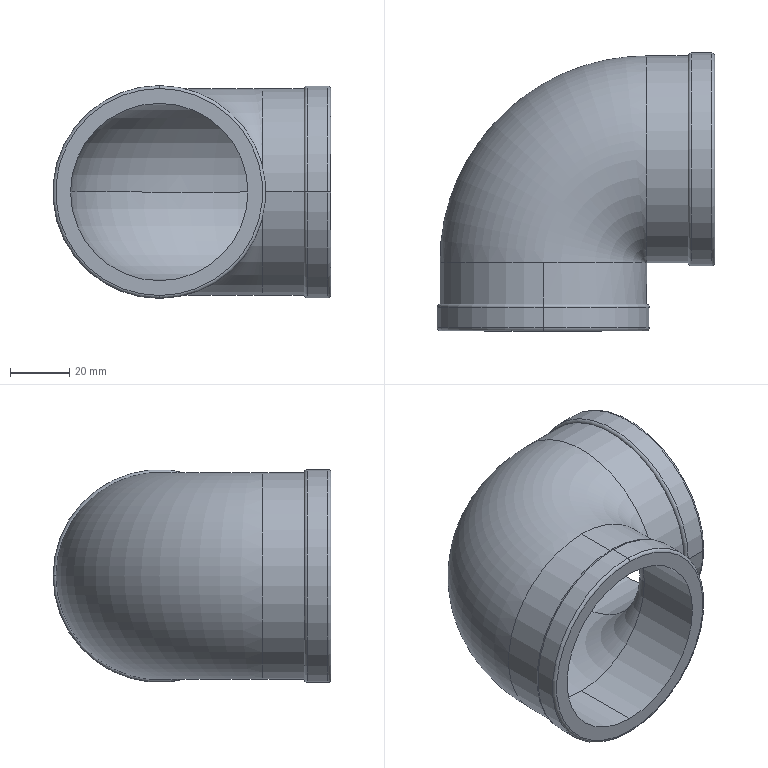Part | SolidWorks | features BossThin 2, Fillet 2, Sweep 1 | 1 solid | 25 faces | box 94 x 94 x 72 mm | volume 106922 mm3 | cylinder 12 | torus 11 | plane 2 | commonest cylinder face diameters 60 x4 70 x4 72 x4
STEP:
#1=CARTESIAN_POINT('',(-30.,23.,0.));
#2=VERTEX_POINT('',#1);
#3=CARTESIAN_POINT('',(0.,23.,30.));
#4=VERTEX_POINT('',#3);
#5=CARTESIAN_POINT('',(0.,23.,0.));
#6=DIRECTION('',(0.,1.,0.));
#7=DIRECTION('',(0.,0.,1.));
#8=AXIS2_PLACEMENT_3D('',#5,#6,#7);
#9=CIRCLE('',#8,30.);
#10=EDGE_CURVE('',#2,#4,#9,.T.);
#11=ORIENTED_EDGE('',*,*,#10,.F.);
#12=CARTESIAN_POINT('',(35.,88.,0.));
#13=VERTEX_POINT('',#12);
#14=CARTESIAN_POINT('',(35.,23.,0.));
#15=DIRECTION('',(0.,0.,-1.));
#16=DIRECTION('',(0.,1.,0.));
#17=AXIS2_PLACEMENT_3D('',#14,#15,#16);
#18=CIRCLE('',#17,65.);
#19=EDGE_CURVE('',#2,#13,#18,.T.);
#20=ORIENTED_EDGE('',*,*,#19,.T.);
#21=CARTESIAN_POINT('',(35.,28.,0.));
#22=VERTEX_POINT('',#21);
#23=CARTESIAN_POINT('',(35.,58.,0.));
#24=DIRECTION('',(1.,0.,0.));
#25=DIRECTION('',(0.,0.,1.));
#26=AXIS2_PLACEMENT_3D('',#23,#24,#25);
#27=CIRCLE('',#26,30.);
#28=EDGE_CURVE('',#13,#22,#27,.T.);
#29=ORIENTED_EDGE('',*,*,#28,.T.);
#30=CARTESIAN_POINT('',(30.,23.,0.));
#31=VERTEX_POINT('',#30);
#32=CARTESIAN_POINT('',(35.,23.,0.));
#33=DIRECTION('',(0.,0.,-1.));
#34=DIRECTION('',(0.,1.,0.));
#35=AXIS2_PLACEMENT_3D('',#32,#33,#34);
#36=CIRCLE('',#35,5.);
#37=EDGE_CURVE('',#31,#22,#36,.T.);
#38=ORIENTED_EDGE('',*,*,#37,.F.);
#39=CARTESIAN_POINT('',(0.,23.,0.));
#40=DIRECTION('',(0.,1.,0.));
#41=DIRECTION('',(0.,0.,1.));
#42=AXIS2_PLACEMENT_3D('',#39,#40,#41);
#43=CIRCLE('',#42,30.);
#44=EDGE_CURVE('',#4,#31,#43,.T.);
#45=ORIENTED_EDGE('',*,*,#44,.F.);
#46=EDGE_LOOP('',(#11,#20,#29,#38,#45));
#47=FACE_OUTER_BOUND('',#46,.T.);
#48=CARTESIAN_POINT('',(35.,23.,0.));
#49=DIRECTION('',(0.,0.,-1.));
#50=DIRECTION('',(-1.,0.,0.));
#51=AXIS2_PLACEMENT_3D('',#48,#49,#50);
#52=TOROIDAL_SURFACE('',#51,35.,30.);
#53=ADVANCED_FACE('',(#47),#52,.F.);
#54=CARTESIAN_POINT('',(57.,22.,0.));
#55=VERTEX_POINT('',#54);
#56=CARTESIAN_POINT('',(57.,94.,0.));
#57=VERTEX_POINT('',#56);
#58=CARTESIAN_POINT('',(57.,58.,0.));
#59=DIRECTION('',(-1.,0.,0.));
#60=DIRECTION('',(0.,1.,0.));
#61=AXIS2_PLACEMENT_3D('',#58,#59,#60);
#62=CIRCLE('',#61,36.);
#63=EDGE_CURVE('',#55,#57,#62,.T.);
#64=ORIENTED_EDGE('',*,*,#63,.F.);
#65=CARTESIAN_POINT('',(58.,23.,0.));
#66=VERTEX_POINT('',#65);
#67=CARTESIAN_POINT('',(57.,23.,0.));
#68=DIRECTION('',(0.,0.,1.));
#69=DIRECTION('',(0.,-1.,0.));
#70=AXIS2_PLACEMENT_3D('',#67,#68,#69);
#71=CIRCLE('',#70,1.);
#72=EDGE_CURVE('',#55,#66,#71,.T.);
#73=ORIENTED_EDGE('',*,*,#72,.T.);
#74=CARTESIAN_POINT('',(58.,93.,0.));
#75=VERTEX_POINT('',#74);
#76=CARTESIAN_POINT('',(58.,58.,0.));
#77=DIRECTION('',(1.,0.,0.));
#78=DIRECTION('',(0.,1.,0.));
#79=AXIS2_PLACEMENT_3D('',#76,#77,#78);
#80=CIRCLE('',#79,35.);
#81=EDGE_CURVE('',#75,#66,#80,.T.);
#82=ORIENTED_EDGE('',*,*,#81,.F.);
#83=CARTESIAN_POINT('',(57.,93.,0.));
#84=DIRECTION('',(0.,0.,-1.));
#85=DIRECTION('',(0.,1.,0.));
#86=AXIS2_PLACEMENT_3D('',#83,#84,#85);
#87=CIRCLE('',#86,1.);
#88=EDGE_CURVE('',#57,#75,#87,.T.);
#89=ORIENTED_EDGE('',*,*,#88,.F.);
#90=EDGE_LOOP('',(#64,#73,#82,#89));
#91=FACE_OUTER_BOUND('',#90,.T.);
#92=CARTESIAN_POINT('',(57.,58.,0.));
#93=DIRECTION('',(1.,0.,0.));
#94=DIRECTION('',(0.,1.,0.));
#95=AXIS2_PLACEMENT_3D('',#92,#93,#94);
#96=TOROIDAL_SURFACE('',#95,35.,1.);
#97=ADVANCED_FACE('',(#91),#96,.T.);
#98=CARTESIAN_POINT('',(49.,93.,0.));
#99=VERTEX_POINT('',#98);
#100=CARTESIAN_POINT('',(49.,23.,0.));
#101=VERTEX_POINT('',#100);
#102=CARTESIAN_POINT('',(49.,58.,0.));
#103=DIRECTION('',(1.,0.,0.));
#104=DIRECTION('',(0.,1.,0.));
#105=AXIS2_PLACEMENT_3D('',#102,#103,#104);
#106=CIRCLE('',#105,35.);
#107=EDGE_CURVE('',#99,#101,#106,.T.);
#108=ORIENTED_EDGE('',*,*,#107,.T.);
#109=CARTESIAN_POINT('',(50.,22.,0.));
#110=VERTEX_POINT('',#109);
#111=CARTESIAN_POINT('',(50.,23.,0.));
#112=DIRECTION('',(0.,0.,1.));
#113=DIRECTION('',(0.,-1.,0.));
#114=AXIS2_PLACEMENT_3D('',#111,#112,#113);
#115=CIRCLE('',#114,1.);
#116=EDGE_CURVE('',#101,#110,#115,.T.);
#117=ORIENTED_EDGE('',*,*,#116,.T.);
#118=CARTESIAN_POINT('',(50.,94.,0.));
#119=VERTEX_POINT('',#118);
#120=CARTESIAN_POINT('',(50.,58.,0.));
#121=DIRECTION('',(1.,0.,0.));
#122=DIRECTION('',(0.,1.,0.));
#123=AXIS2_PLACEMENT_3D('',#120,#121,#122);
#124=CIRCLE('',#123,36.);
#125=EDGE_CURVE('',#119,#110,#124,.T.);
#126=ORIENTED_EDGE('',*,*,#125,.F.);
#127=CARTESIAN_POINT('',(50.,93.,0.));
#128=DIRECTION('',(0.,0.,-1.));
#129=DIRECTION('',(0.,1.,0.));
#130=AXIS2_PLACEMENT_3D('',#127,#128,#129);
#131=CIRCLE('',#130,1.);
#132=EDGE_CURVE('',#99,#119,#131,.T.);
#133=ORIENTED_EDGE('',*,*,#132,.F.);
#134=EDGE_LOOP('',(#108,#117,#126,#133));
#135=FACE_OUTER_BOUND('',#134,.T.);
#136=CARTESIAN_POINT('',(50.,58.,0.));
#137=DIRECTION('',(1.,0.,0.));
#138=DIRECTION('',(0.,1.,0.));
#139=AXIS2_PLACEMENT_3D('',#136,#137,#138);
#140=TOROIDAL_SURFACE('',#139,35.,1.);
#141=ADVANCED_FACE('',(#135),#140,.T.);
#142=ORIENTED_EDGE('',*,*,#125,.T.);
#143=CARTESIAN_POINT('',(49.,22.,0.));
#144=DIRECTION('',(1.,0.,0.));
#145=VECTOR('',#144,1000.);
#146=LINE('',#143,#145);
#147=EDGE_CURVE('',#110,#55,#146,.T.);
#148=ORIENTED_EDGE('',*,*,#147,.T.);
#149=ORIENTED_EDGE('',*,*,#63,.T.);
#150=CARTESIAN_POINT('',(49.,94.,0.));
#151=DIRECTION('',(1.,0.,0.));
#152=VECTOR('',#151,1000.);
#153=LINE('',#150,#152);
#154=EDGE_CURVE('',#119,#57,#153,.T.);
#155=ORIENTED_EDGE('',*,*,#154,.F.);
#156=EDGE_LOOP('',(#142,#148,#149,#155));
#157=FACE_OUTER_BOUND('',#156,.T.);
#158=CARTESIAN_POINT('',(49.,58.,0.));
#159=DIRECTION('',(1.,0.,0.));
#160=DIRECTION('',(0.,1.,0.));
#161=AXIS2_PLACEMENT_3D('',#158,#159,#160);
#162=CYLINDRICAL_SURFACE('',#161,36.);
#163=ADVANCED_FACE('',(#157),#162,.T.);
#164=CARTESIAN_POINT('',(0.,0.,-35.));
#165=VERTEX_POINT('',#164);
#166=CARTESIAN_POINT('',(0.,0.,35.));
#167=VERTEX_POINT('',#166);
#168=CARTESIAN_POINT('',(0.,0.,0.));
#169=DIRECTION('',(0.,-1.,0.));
#170=DIRECTION('',(0.,0.,1.));
#171=AXIS2_PLACEMENT_3D('',#168,#169,#170);
#172=CIRCLE('',#171,35.);
#173=EDGE_CURVE('',#165,#167,#172,.T.);
#174=ORIENTED_EDGE('',*,*,#173,.F.);
#175=CARTESIAN_POINT('',(0.,1.,-36.));
#176=VERTEX_POINT('',#175);
#177=CARTESIAN_POINT('',(0.,1.,-35.));
#178=DIRECTION('',(1.,0.,0.));
#179=DIRECTION('',(0.,0.,-1.));
#180=AXIS2_PLACEMENT_3D('',#177,#178,#179);
#181=CIRCLE('',#180,1.);
#182=EDGE_CURVE('',#165,#176,#181,.T.);
#183=ORIENTED_EDGE('',*,*,#182,.T.);
#184=CARTESIAN_POINT('',(0.,1.,36.));
#185=VERTEX_POINT('',#184);
#186=CARTESIAN_POINT('',(0.,1.,0.));
#187=DIRECTION('',(0.,1.,0.));
#188=DIRECTION('',(0.,0.,1.));
#189=AXIS2_PLACEMENT_3D('',#186,#187,#188);
#190=CIRCLE('',#189,36.);
#191=EDGE_CURVE('',#185,#176,#190,.T.);
#192=ORIENTED_EDGE('',*,*,#191,.F.);
#193=CARTESIAN_POINT('',(0.,1.,35.));
#194=DIRECTION('',(-1.,0.,0.));
#195=DIRECTION('',(0.,0.,1.));
#196=AXIS2_PLACEMENT_3D('',#193,#194,#195);
#197=CIRCLE('',#196,1.);
#198=EDGE_CURVE('',#167,#185,#197,.T.);
#199=ORIENTED_EDGE('',*,*,#198,.F.);
#200=EDGE_LOOP('',(#174,#183,#192,#199));
#201=FACE_OUTER_BOUND('',#200,.T.);
#202=CARTESIAN_POINT('',(0.,1.,0.));
#203=DIRECTION('',(0.,1.,0.));
#204=DIRECTION('',(0.,0.,1.));
#205=AXIS2_PLACEMENT_3D('',#202,#203,#204);
#206=TOROIDAL_SURFACE('',#205,35.,1.);
#207=ADVANCED_FACE('',(#201),#206,.T.);
#208=CARTESIAN_POINT('',(0.,9.,-35.));
#209=VERTEX_POINT('',#208);
#210=CARTESIAN_POINT('',(0.,9.,35.));
#211=VERTEX_POINT('',#210);
#212=CARTESIAN_POINT('',(0.,9.,0.));
#213=DIRECTION('',(0.,-1.,0.));
#214=DIRECTION('',(0.,0.,-1.));
#215=AXIS2_PLACEMENT_3D('',#212,#213,#214);
#216=CIRCLE('',#215,35.);
#217=EDGE_CURVE('',#209,#211,#216,.T.);
#218=ORIENTED_EDGE('',*,*,#217,.T.);
#219=CARTESIAN_POINT('',(0.,8.,36.));
#220=VERTEX_POINT('',#219);
#221=CARTESIAN_POINT('',(0.,8.,35.));
#222=DIRECTION('',(1.,0.,0.));
#223=DIRECTION('',(0.,0.,-1.));
#224=AXIS2_PLACEMENT_3D('',#221,#222,#223);
#225=CIRCLE('',#224,1.);
#226=EDGE_CURVE('',#211,#220,#225,.T.);
#227=ORIENTED_EDGE('',*,*,#226,.T.);
#228=CARTESIAN_POINT('',(0.,8.,-36.));
#229=VERTEX_POINT('',#228);
#230=CARTESIAN_POINT('',(0.,8.,0.));
#231=DIRECTION('',(0.,-1.,0.));
#232=DIRECTION('',(0.,0.,-1.));
#233=AXIS2_PLACEMENT_3D('',#230,#231,#232);
#234=CIRCLE('',#233,36.);
#235=EDGE_CURVE('',#229,#220,#234,.T.);
#236=ORIENTED_EDGE('',*,*,#235,.F.);
#237=CARTESIAN_POINT('',(0.,8.,-35.));
#238=DIRECTION('',(-1.,0.,0.));
#239=DIRECTION('',(0.,0.,1.));
#240=AXIS2_PLACEMENT_3D('',#237,#238,#239);
#241=CIRCLE('',#240,1.);
#242=EDGE_CURVE('',#209,#229,#241,.T.);
#243=ORIENTED_EDGE('',*,*,#242,.F.);
#244=EDGE_LOOP('',(#218,#227,#236,#243));
#245=FACE_OUTER_BOUND('',#244,.T.);
#246=CARTESIAN_POINT('',(0.,8.,0.));
#247=DIRECTION('',(0.,-1.,0.));
#248=DIRECTION('',(0.,0.,-1.));
#249=AXIS2_PLACEMENT_3D('',#246,#247,#248);
#250=TOROIDAL_SURFACE('',#249,35.,1.);
#251=ADVANCED_FACE('',(#245),#250,.T.);
#252=ORIENTED_EDGE('',*,*,#235,.T.);
#253=CARTESIAN_POINT('',(0.,9.,36.));
#254=DIRECTION('',(0.,-1.,0.));
#255=VECTOR('',#254,1000.);
#256=LINE('',#253,#255);
#257=EDGE_CURVE('',#220,#185,#256,.T.);
#258=ORIENTED_EDGE('',*,*,#257,.T.);
#259=ORIENTED_EDGE('',*,*,#191,.T.);
#260=CARTESIAN_POINT('',(0.,9.,-36.));
#261=DIRECTION('',(0.,-1.,0.));
#262=VECTOR('',#261,1000.);
#263=LINE('',#260,#262);
#264=EDGE_CURVE('',#229,#176,#263,.T.);
#265=ORIENTED_EDGE('',*,*,#264,.F.);
#266=EDGE_LOOP('',(#252,#258,#259,#265));
#267=FACE_OUTER_BOUND('',#266,.T.);
#268=CARTESIAN_POINT('',(0.,9.,0.));
#269=DIRECTION('',(0.,-1.,0.));
#270=DIRECTION('',(0.,0.,-1.));
#271=AXIS2_PLACEMENT_3D('',#268,#269,#270);
#272=CYLINDRICAL_SURFACE('',#271,36.);
#273=ADVANCED_FACE('',(#267),#272,.T.);
#274=CARTESIAN_POINT('',(0.,23.,-30.));
#275=VERTEX_POINT('',#274);
#276=CARTESIAN_POINT('',(0.,23.,0.));
#277=DIRECTION('',(0.,1.,0.));
#278=DIRECTION('',(0.,0.,1.));
#279=AXIS2_PLACEMENT_3D('',#276,#277,#278);
#280=CIRCLE('',#279,30.);
#281=EDGE_CURVE('',#275,#2,#280,.T.);
#282=ORIENTED_EDGE('',*,*,#281,.T.);
#283=ORIENTED_EDGE('',*,*,#10,.T.);
#284=CARTESIAN_POINT('',(0.,0.,30.));
#285=VERTEX_POINT('',#284);
#286=CARTESIAN_POINT('',(0.,23.,30.));
#287=DIRECTION('',(0.,-1.,0.));
#288=VECTOR('',#287,1000.);
#289=LINE('',#286,#288);
#290=EDGE_CURVE('',#4,#285,#289,.T.);
#291=ORIENTED_EDGE('',*,*,#290,.T.);
#292=CARTESIAN_POINT('',(0.,0.,-30.));
#293=VERTEX_POINT('',#292);
#294=CARTESIAN_POINT('',(0.,0.,0.));
#295=DIRECTION('',(0.,1.,0.));
#296=DIRECTION('',(0.,0.,1.));
#297=AXIS2_PLACEMENT_3D('',#294,#295,#296);
#298=CIRCLE('',#297,30.);
#299=EDGE_CURVE('',#293,#285,#298,.T.);
#300=ORIENTED_EDGE('',*,*,#299,.F.);
#301=CARTESIAN_POINT('',(0.,23.,-30.));
#302=DIRECTION('',(0.,-1.,0.));
#303=VECTOR('',#302,1000.);
#304=LINE('',#301,#303);
#305=EDGE_CURVE('',#275,#293,#304,.T.);
#306=ORIENTED_EDGE('',*,*,#305,.F.);
#307=EDGE_LOOP('',(#282,#283,#291,#300,#306));
#308=FACE_OUTER_BOUND('',#307,.T.);
#309=CARTESIAN_POINT('',(0.,23.,0.));
#310=DIRECTION('',(0.,-1.,0.));
#311=DIRECTION('',(0.,0.,-1.));
#312=AXIS2_PLACEMENT_3D('',#309,#310,#311);
#313=CYLINDRICAL_SURFACE('',#312,30.);
#314=ADVANCED_FACE('',(#308),#313,.F.);
#315=CARTESIAN_POINT('',(35.,58.,0.));
#316=DIRECTION('',(1.,0.,0.));
#317=DIRECTION('',(0.,0.,1.));
#318=AXIS2_PLACEMENT_3D('',#315,#316,#317);
#319=CIRCLE('',#318,30.);
#320=EDGE_CURVE('',#22,#13,#319,.T.);
#321=ORIENTED_EDGE('',*,*,#320,.F.);
#322=CARTESIAN_POINT('',(58.,28.,0.));
#323=VERTEX_POINT('',#322);
#324=CARTESIAN_POINT('',(35.,28.,0.));
#325=DIRECTION('',(1.,0.,0.));
#326=VECTOR('',#325,1000.);
#327=LINE('',#324,#326);
#328=EDGE_CURVE('',#22,#323,#327,.T.);
#329=ORIENTED_EDGE('',*,*,#328,.T.);
#330=CARTESIAN_POINT('',(58.,88.,0.));
#331=VERTEX_POINT('',#330);
#332=CARTESIAN_POINT('',(58.,58.,0.));
#333=DIRECTION('',(1.,0.,0.));
#334=DIRECTION('',(0.,0.,1.));
#335=AXIS2_PLACEMENT_3D('',#332,#333,#334);
#336=CIRCLE('',#335,30.);
#337=EDGE_CURVE('',#323,#331,#336,.T.);
#338=ORIENTED_EDGE('',*,*,#337,.T.);
#339=CARTESIAN_POINT('',(35.,88.,0.));
#340=DIRECTION('',(1.,0.,0.));
#341=VECTOR('',#340,1000.);
#342=LINE('',#339,#341);
#343=EDGE_CURVE('',#13,#331,#342,.T.);
#344=ORIENTED_EDGE('',*,*,#343,.F.);
#345=EDGE_LOOP('',(#321,#329,#338,#344));
#346=FACE_OUTER_BOUND('',#345,.T.);
#347=CARTESIAN_POINT('',(35.,58.,0.));
#348=DIRECTION('',(1.,0.,0.));
#349=DIRECTION('',(0.,1.,0.));
#350=AXIS2_PLACEMENT_3D('',#347,#348,#349);
#351=CYLINDRICAL_SURFACE('',#350,30.);
#352=ADVANCED_FACE('',(#346),#351,.F.);
#353=CARTESIAN_POINT('',(0.,23.,35.));
#354=VERTEX_POINT('',#353);
#355=CARTESIAN_POINT('',(35.,23.,0.));
#356=VERTEX_POINT('',#355);
#357=CARTESIAN_POINT('',(0.,23.,0.));
#358=DIRECTION('',(0.,1.,0.));
#359=DIRECTION('',(0.,0.,1.));
#360=AXIS2_PLACEMENT_3D('',#357,#358,#359);
#361=CIRCLE('',#360,35.);
#362=EDGE_CURVE('',#354,#356,#361,.T.);
#363=ORIENTED_EDGE('',*,*,#362,.F.);
#364=CARTESIAN_POINT('',(0.,23.,35.));
#365=DIRECTION('',(0.,-1.,0.));
#366=VECTOR('',#365,1000.);
#367=LINE('',#364,#366);
#368=EDGE_CURVE('',#354,#211,#367,.T.);
#369=ORIENTED_EDGE('',*,*,#368,.T.);
#370=ORIENTED_EDGE('',*,*,#217,.F.);
#371=CARTESIAN_POINT('',(0.,23.,-35.));
#372=VERTEX_POINT('',#371);
#373=CARTESIAN_POINT('',(0.,23.,-35.));
#374=DIRECTION('',(0.,-1.,0.));
#375=VECTOR('',#374,1000.);
#376=LINE('',#373,#375);
#377=EDGE_CURVE('',#372,#209,#376,.T.);
#378=ORIENTED_EDGE('',*,*,#377,.F.);
#379=CARTESIAN_POINT('',(0.,23.,0.));
#380=DIRECTION('',(0.,1.,0.));
#381=DIRECTION('',(0.,0.,1.));
#382=AXIS2_PLACEMENT_3D('',#379,#380,#381);
#383=CIRCLE('',#382,35.);
#384=EDGE_CURVE('',#356,#372,#383,.T.);
#385=ORIENTED_EDGE('',*,*,#384,.F.);
#386=EDGE_LOOP('',(#363,#369,#370,#378,#385));
#387=FACE_OUTER_BOUND('',#386,.T.);
#388=CARTESIAN_POINT('',(0.,23.,0.));
#389=DIRECTION('',(0.,-1.,0.));
#390=DIRECTION('',(0.,0.,-1.));
#391=AXIS2_PLACEMENT_3D('',#388,#389,#390);
#392=CYLINDRICAL_SURFACE('',#391,35.);
#393=ADVANCED_FACE('',(#387),#392,.T.);
#394=CARTESIAN_POINT('',(35.,93.,0.));
#395=VERTEX_POINT('',#394);
#396=CARTESIAN_POINT('',(35.,58.,0.));
#397=DIRECTION('',(1.,0.,0.));
#398=DIRECTION('',(0.,0.,1.));
#399=AXIS2_PLACEMENT_3D('',#396,#397,#398);
#400=CIRCLE('',#399,35.);
#401=EDGE_CURVE('',#395,#356,#400,.T.);
#402=ORIENTED_EDGE('',*,*,#401,.T.);
#403=CARTESIAN_POINT('',(35.,23.,0.));
#404=DIRECTION('',(1.,0.,0.));
#405=VECTOR('',#404,1000.);
#406=LINE('',#403,#405);
#407=EDGE_CURVE('',#356,#101,#406,.T.);
#408=ORIENTED_EDGE('',*,*,#407,.T.);
#409=ORIENTED_EDGE('',*,*,#107,.F.);
#410=CARTESIAN_POINT('',(35.,93.,0.));
#411=DIRECTION('',(1.,0.,0.));
#412=VECTOR('',#411,1000.);
#413=LINE('',#410,#412);
#414=EDGE_CURVE('',#395,#99,#413,.T.);
#415=ORIENTED_EDGE('',*,*,#414,.F.);
#416=EDGE_LOOP('',(#402,#408,#409,#415));
#417=FACE_OUTER_BOUND('',#416,.T.);
#418=CARTESIAN_POINT('',(35.,58.,0.));
#419=DIRECTION('',(1.,0.,0.));
#420=DIRECTION('',(0.,1.,0.));
#421=AXIS2_PLACEMENT_3D('',#418,#419,#420);
#422=CYLINDRICAL_SURFACE('',#421,35.);
#423=ADVANCED_FACE('',(#417),#422,.T.);
#424=ORIENTED_EDGE('',*,*,#407,.F.);
#425=CARTESIAN_POINT('',(35.,58.,0.));
#426=DIRECTION('',(1.,0.,0.));
#427=DIRECTION('',(0.,0.,1.));
#428=AXIS2_PLACEMENT_3D('',#425,#426,#427);
#429=CIRCLE('',#428,35.);
#430=EDGE_CURVE('',#356,#395,#429,.T.);
#431=ORIENTED_EDGE('',*,*,#430,.T.);
#432=ORIENTED_EDGE('',*,*,#414,.T.);
#433=CARTESIAN_POINT('',(49.,58.,0.));
#434=DIRECTION('',(1.,0.,0.));
#435=DIRECTION('',(0.,1.,0.));
#436=AXIS2_PLACEMENT_3D('',#433,#434,#435);
#437=CIRCLE('',#436,35.);
#438=EDGE_CURVE('',#101,#99,#437,.T.);
#439=ORIENTED_EDGE('',*,*,#438,.F.);
#440=EDGE_LOOP('',(#424,#431,#432,#439));
#441=FACE_OUTER_BOUND('',#440,.T.);
#442=CARTESIAN_POINT('',(35.,58.,0.));
#443=DIRECTION('',(1.,0.,0.));
#444=DIRECTION('',(0.,1.,0.));
#445=AXIS2_PLACEMENT_3D('',#442,#443,#444);
#446=CYLINDRICAL_SURFACE('',#445,35.);
#447=ADVANCED_FACE('',(#441),#446,.T.);
#448=ORIENTED_EDGE('',*,*,#368,.F.);
#449=CARTESIAN_POINT('',(0.,23.,0.));
#450=DIRECTION('',(0.,1.,0.));
#451=DIRECTION('',(0.,0.,1.));
#452=AXIS2_PLACEMENT_3D('',#449,#450,#451);
#453=CIRCLE('',#452,35.);
#454=EDGE_CURVE('',#372,#354,#453,.T.);
#455=ORIENTED_EDGE('',*,*,#454,.F.);
#456=ORIENTED_EDGE('',*,*,#377,.T.);
#457=CARTESIAN_POINT('',(0.,9.,0.));
#458=DIRECTION('',(0.,-1.,0.));
#459=DIRECTION('',(0.,0.,-1.));
#460=AXIS2_PLACEMENT_3D('',#457,#458,#459);
#461=CIRCLE('',#460,35.);
#462=EDGE_CURVE('',#211,#209,#461,.T.);
#463=ORIENTED_EDGE('',*,*,#462,.F.);
#464=EDGE_LOOP('',(#448,#455,#456,#463));
#465=FACE_OUTER_BOUND('',#464,.T.);
#466=CARTESIAN_POINT('',(0.,23.,0.));
#467=DIRECTION('',(0.,-1.,0.));
#468=DIRECTION('',(0.,0.,-1.));
#469=AXIS2_PLACEMENT_3D('',#466,#467,#468);
#470=CYLINDRICAL_SURFACE('',#469,35.);
#471=ADVANCED_FACE('',(#465),#470,.T.);
#472=ORIENTED_EDGE('',*,*,#328,.F.);
#473=ORIENTED_EDGE('',*,*,#28,.F.);
#474=ORIENTED_EDGE('',*,*,#343,.T.);
#475=CARTESIAN_POINT('',(58.,58.,0.));
#476=DIRECTION('',(1.,0.,0.));
#477=DIRECTION('',(0.,0.,1.));
#478=AXIS2_PLACEMENT_3D('',#475,#476,#477);
#479=CIRCLE('',#478,30.);
#480=EDGE_CURVE('',#331,#323,#479,.T.);
#481=ORIENTED_EDGE('',*,*,#480,.T.);
#482=EDGE_LOOP('',(#472,#473,#474,#481));
#483=FACE_OUTER_BOUND('',#482,.T.);
#484=CARTESIAN_POINT('',(35.,58.,0.));
#485=DIRECTION('',(1.,0.,0.));
#486=DIRECTION('',(0.,1.,0.));
#487=AXIS2_PLACEMENT_3D('',#484,#485,#486);
#488=CYLINDRICAL_SURFACE('',#487,30.);
#489=ADVANCED_FACE('',(#483),#488,.F.);
#490=ORIENTED_EDGE('',*,*,#384,.T.);
#491=ORIENTED_EDGE('',*,*,#454,.T.);
#492=ORIENTED_EDGE('',*,*,#362,.T.);
#493=ORIENTED_EDGE('',*,*,#401,.F.);
#494=ORIENTED_EDGE('',*,*,#430,.F.);
#495=EDGE_LOOP('',(#490,#491,#492,#493,#494));
#496=FACE_OUTER_BOUND('',#495,.T.);
#497=CARTESIAN_POINT('',(35.,23.,0.));
#498=DIRECTION('',(0.,0.,-1.));
#499=DIRECTION('',(-1.,0.,0.));
#500=AXIS2_PLACEMENT_3D('',#497,#498,#499);
#501=TOROIDAL_SURFACE('',#500,35.,35.);
#502=ADVANCED_FACE('',(#496),#501,.T.);
#503=ORIENTED_EDGE('',*,*,#19,.F.);
#504=ORIENTED_EDGE('',*,*,#281,.F.);
#505=CARTESIAN_POINT('',(0.,23.,0.));
#506=DIRECTION('',(0.,1.,0.));
#507=DIRECTION('',(0.,0.,1.));
#508=AXIS2_PLACEMENT_3D('',#505,#506,#507);
#509=CIRCLE('',#508,30.);
#510=EDGE_CURVE('',#31,#275,#509,.T.);
#511=ORIENTED_EDGE('',*,*,#510,.F.);
#512=ORIENTED_EDGE('',*,*,#37,.T.);
#513=ORIENTED_EDGE('',*,*,#320,.T.);
#514=EDGE_LOOP('',(#503,#504,#511,#512,#513));
#515=FACE_OUTER_BOUND('',#514,.T.);
#516=CARTESIAN_POINT('',(35.,23.,0.));
#517=DIRECTION('',(0.,0.,-1.));
#518=DIRECTION('',(-1.,0.,0.));
#519=AXIS2_PLACEMENT_3D('',#516,#517,#518);
#520=TOROIDAL_SURFACE('',#519,35.,30.);
#521=ADVANCED_FACE('',(#515),#520,.F.);
#522=ORIENTED_EDGE('',*,*,#290,.F.);
#523=ORIENTED_EDGE('',*,*,#44,.T.);
#524=ORIENTED_EDGE('',*,*,#510,.T.);
#525=ORIENTED_EDGE('',*,*,#305,.T.);
#526=CARTESIAN_POINT('',(0.,0.,0.));
#527=DIRECTION('',(0.,1.,0.));
#528=DIRECTION('',(0.,0.,1.));
#529=AXIS2_PLACEMENT_3D('',#526,#527,#528);
#530=CIRCLE('',#529,30.);
#531=EDGE_CURVE('',#285,#293,#530,.T.);
#532=ORIENTED_EDGE('',*,*,#531,.F.);
#533=EDGE_LOOP('',(#522,#523,#524,#525,#532));
#534=FACE_OUTER_BOUND('',#533,.T.);
#535=CARTESIAN_POINT('',(0.,23.,0.));
#536=DIRECTION('',(0.,-1.,0.));
#537=DIRECTION('',(0.,0.,-1.));
#538=AXIS2_PLACEMENT_3D('',#535,#536,#537);
#539=CYLINDRICAL_SURFACE('',#538,30.);
#540=ADVANCED_FACE('',(#534),#539,.F.);
#541=ORIENTED_EDGE('',*,*,#81,.T.);
#542=CARTESIAN_POINT('',(58.,58.,0.));
#543=DIRECTION('',(1.,0.,0.));
#544=DIRECTION('',(0.,1.,0.));
#545=AXIS2_PLACEMENT_3D('',#542,#543,#544);
#546=CIRCLE('',#545,35.);
#547=EDGE_CURVE('',#66,#75,#546,.T.);
#548=ORIENTED_EDGE('',*,*,#547,.T.);
#549=EDGE_LOOP('',(#541,#548));
#550=FACE_OUTER_BOUND('',#549,.T.);
#551=ORIENTED_EDGE('',*,*,#480,.F.);
#552=ORIENTED_EDGE('',*,*,#337,.F.);
#553=EDGE_LOOP('',(#551,#552));
#554=FACE_BOUND('',#553,.T.);
#555=CARTESIAN_POINT('',(58.,58.,0.));
#556=DIRECTION('',(1.,0.,0.));
#557=DIRECTION('',(0.,0.,1.));
#558=AXIS2_PLACEMENT_3D('',#555,#556,#557);
#559=PLANE('',#558);
#560=ADVANCED_FACE('',(#550,#554),#559,.T.);
#561=CARTESIAN_POINT('',(0.,0.,0.));
#562=DIRECTION('',(0.,-1.,0.));
#563=DIRECTION('',(0.,0.,1.));
#564=AXIS2_PLACEMENT_3D('',#561,#562,#563);
#565=CIRCLE('',#564,35.);
#566=EDGE_CURVE('',#167,#165,#565,.T.);
#567=ORIENTED_EDGE('',*,*,#566,.T.);
#568=ORIENTED_EDGE('',*,*,#173,.T.);
#569=EDGE_LOOP('',(#567,#568));
#570=FACE_OUTER_BOUND('',#569,.T.);
#571=ORIENTED_EDGE('',*,*,#299,.T.);
#572=ORIENTED_EDGE('',*,*,#531,.T.);
#573=EDGE_LOOP('',(#571,#572));
#574=FACE_BOUND('',#573,.T.);
#575=CARTESIAN_POINT('',(0.,0.,0.));
#576=DIRECTION('',(0.,1.,0.));
#577=DIRECTION('',(0.,0.,1.));
#578=AXIS2_PLACEMENT_3D('',#575,#576,#577);
#579=PLANE('',#578);
#580=ADVANCED_FACE('',(#570,#574),#579,.F.);
#581=ORIENTED_EDGE('',*,*,#257,.F.);
#582=CARTESIAN_POINT('',(0.,8.,0.));
#583=DIRECTION('',(0.,-1.,0.));
#584=DIRECTION('',(0.,0.,-1.));
#585=AXIS2_PLACEMENT_3D('',#582,#583,#584);
#586=CIRCLE('',#585,36.);
#587=EDGE_CURVE('',#220,#229,#586,.T.);
#588=ORIENTED_EDGE('',*,*,#587,.T.);
#589=ORIENTED_EDGE('',*,*,#264,.T.);
#590=CARTESIAN_POINT('',(0.,1.,0.));
#591=DIRECTION('',(0.,1.,0.));
#592=DIRECTION('',(0.,0.,1.));
#593=AXIS2_PLACEMENT_3D('',#590,#591,#592);
#594=CIRCLE('',#593,36.);
#595=EDGE_CURVE('',#176,#185,#594,.T.);
#596=ORIENTED_EDGE('',*,*,#595,.T.);
#597=EDGE_LOOP('',(#581,#588,#589,#596));
#598=FACE_OUTER_BOUND('',#597,.T.);
#599=CARTESIAN_POINT('',(0.,9.,0.));
#600=DIRECTION('',(0.,-1.,0.));
#601=DIRECTION('',(0.,0.,-1.));
#602=AXIS2_PLACEMENT_3D('',#599,#600,#601);
#603=CYLINDRICAL_SURFACE('',#602,36.);
#604=ADVANCED_FACE('',(#598),#603,.T.);
#605=ORIENTED_EDGE('',*,*,#226,.F.);
#606=ORIENTED_EDGE('',*,*,#462,.T.);
#607=ORIENTED_EDGE('',*,*,#242,.T.);
#608=ORIENTED_EDGE('',*,*,#587,.F.);
#609=EDGE_LOOP('',(#605,#606,#607,#608));
#610=FACE_OUTER_BOUND('',#609,.T.);
#611=CARTESIAN_POINT('',(0.,8.,0.));
#612=DIRECTION('',(0.,-1.,0.));
#613=DIRECTION('',(0.,0.,-1.));
#614=AXIS2_PLACEMENT_3D('',#611,#612,#613);
#615=TOROIDAL_SURFACE('',#614,35.,1.);
#616=ADVANCED_FACE('',(#610),#615,.T.);
#617=ORIENTED_EDGE('',*,*,#182,.F.);
#618=ORIENTED_EDGE('',*,*,#566,.F.);
#619=ORIENTED_EDGE('',*,*,#198,.T.);
#620=ORIENTED_EDGE('',*,*,#595,.F.);
#621=EDGE_LOOP('',(#617,#618,#619,#620));
#622=FACE_OUTER_BOUND('',#621,.T.);
#623=CARTESIAN_POINT('',(0.,1.,0.));
#624=DIRECTION('',(0.,1.,0.));
#625=DIRECTION('',(0.,0.,1.));
#626=AXIS2_PLACEMENT_3D('',#623,#624,#625);
#627=TOROIDAL_SURFACE('',#626,35.,1.);
#628=ADVANCED_FACE('',(#622),#627,.T.);
#629=ORIENTED_EDGE('',*,*,#147,.F.);
#630=CARTESIAN_POINT('',(50.,58.,0.));
#631=DIRECTION('',(1.,0.,0.));
#632=DIRECTION('',(0.,1.,0.));
#633=AXIS2_PLACEMENT_3D('',#630,#631,#632);
#634=CIRCLE('',#633,36.);
#635=EDGE_CURVE('',#110,#119,#634,.T.);
#636=ORIENTED_EDGE('',*,*,#635,.T.);
#637=ORIENTED_EDGE('',*,*,#154,.T.);
#638=CARTESIAN_POINT('',(57.,58.,0.));
#639=DIRECTION('',(-1.,0.,0.));
#640=DIRECTION('',(0.,1.,0.));
#641=AXIS2_PLACEMENT_3D('',#638,#639,#640);
#642=CIRCLE('',#641,36.);
#643=EDGE_CURVE('',#57,#55,#642,.T.);
#644=ORIENTED_EDGE('',*,*,#643,.T.);
#645=EDGE_LOOP('',(#629,#636,#637,#644));
#646=FACE_OUTER_BOUND('',#645,.T.);
#647=CARTESIAN_POINT('',(49.,58.,0.));
#648=DIRECTION('',(1.,0.,0.));
#649=DIRECTION('',(0.,1.,0.));
#650=AXIS2_PLACEMENT_3D('',#647,#648,#649);
#651=CYLINDRICAL_SURFACE('',#650,36.);
#652=ADVANCED_FACE('',(#646),#651,.T.);
#653=ORIENTED_EDGE('',*,*,#116,.F.);
#654=ORIENTED_EDGE('',*,*,#438,.T.);
#655=ORIENTED_EDGE('',*,*,#132,.T.);
#656=ORIENTED_EDGE('',*,*,#635,.F.);
#657=EDGE_LOOP('',(#653,#654,#655,#656));
#658=FACE_OUTER_BOUND('',#657,.T.);
#659=CARTESIAN_POINT('',(50.,58.,0.));
#660=DIRECTION('',(1.,0.,0.));
#661=DIRECTION('',(0.,1.,0.));
#662=AXIS2_PLACEMENT_3D('',#659,#660,#661);
#663=TOROIDAL_SURFACE('',#662,35.,1.);
#664=ADVANCED_FACE('',(#658),#663,.T.);
#665=ORIENTED_EDGE('',*,*,#72,.F.);
#666=ORIENTED_EDGE('',*,*,#643,.F.);
#667=ORIENTED_EDGE('',*,*,#88,.T.);
#668=ORIENTED_EDGE('',*,*,#547,.F.);
#669=EDGE_LOOP('',(#665,#666,#667,#668));
#670=FACE_OUTER_BOUND('',#669,.T.);
#671=CARTESIAN_POINT('',(57.,58.,0.));
#672=DIRECTION('',(1.,0.,0.));
#673=DIRECTION('',(0.,1.,0.));
#674=AXIS2_PLACEMENT_3D('',#671,#672,#673);
#675=TOROIDAL_SURFACE('',#674,35.,1.);
#676=ADVANCED_FACE('',(#670),#675,.T.);
#677=CLOSED_SHELL('',(#53,#97,#141,#163,#207,#251,#273,#314,#352,#393,#423,#447,#471,#489,#502,#521,#540,#560,#580,#604,#616,#628,#652,#664,#676));
#678=MANIFOLD_SOLID_BREP('',#677);
#679=CARTESIAN_POINT('',(0.,0.,0.));
#680=DIRECTION('',(0.,0.,1.));
#681=DIRECTION('',(1.,0.,0.));
#682=AXIS2_PLACEMENT_3D('',#679,#680,#681);
#683=(LENGTH_UNIT()NAMED_UNIT(*)SI_UNIT(.MILLI.,.METRE.));
#684=UNCERTAINTY_MEASURE_WITH_UNIT(LENGTH_MEASURE(0.00001),#683,'','');
#685=(NAMED_UNIT(*)PLANE_ANGLE_UNIT()SI_UNIT($,.RADIAN.));
#686=(NAMED_UNIT(*)SI_UNIT($,.STERADIAN.)SOLID_ANGLE_UNIT());
#687=(GEOMETRIC_REPRESENTATION_CONTEXT(3)GLOBAL_UNCERTAINTY_ASSIGNED_CONTEXT((#684))GLOBAL_UNIT_ASSIGNED_CONTEXT((#683,#685,#686))REPRESENTATION_CONTEXT('',''));
#688=ADVANCED_BREP_SHAPE_REPRESENTATION('',(#678,#682),#687);